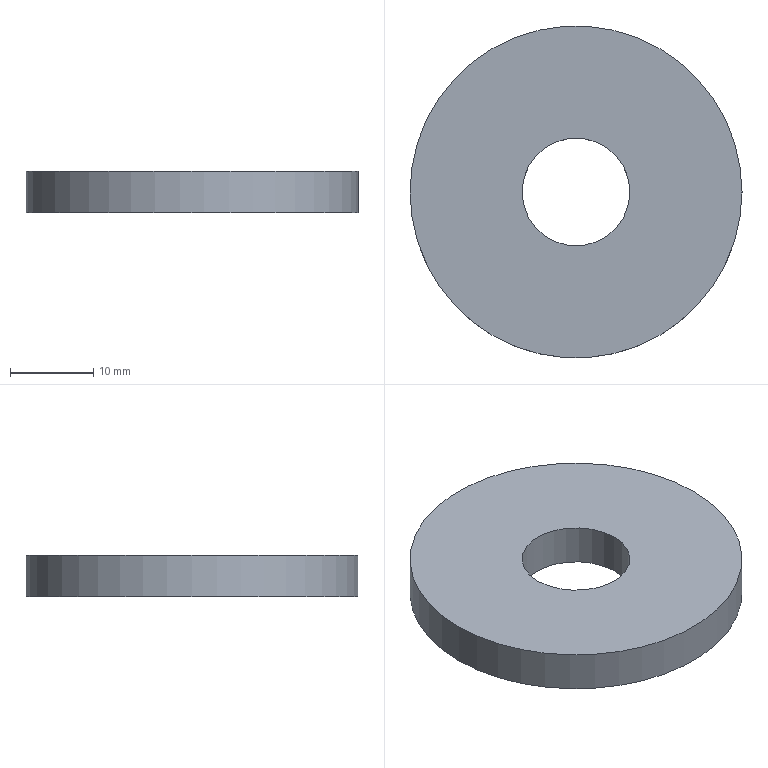Part | NX | features solid 2 | 1 solid | 4 faces | box 40 x 40 x 5 mm | volume 5620 mm3 | plane 2 | cylinder 2 | commonest cylinder face diameters 13 x1 40 x1
STEP:
#1=CARTESIAN_POINT('',(-97.5,-240.,380.));
#2=VERTEX_POINT('',#1);
#3=CARTESIAN_POINT('',(-117.5,-240.,380.));
#4=DIRECTION('',(0.,0.,1.));
#5=DIRECTION('',(1.,0.,0.));
#6=AXIS2_PLACEMENT_3D('',#3,#4,#5);
#7=CIRCLE('',#6,20.);
#8=EDGE_CURVE('',#2,#2,#7,.F.);
#9=ORIENTED_EDGE('',*,*,#8,.F.);
#10=EDGE_LOOP('',(#9));
#11=FACE_BOUND('',#10,.T.);
#12=CARTESIAN_POINT('',(-111.,-240.,380.));
#13=VERTEX_POINT('',#12);
#14=CARTESIAN_POINT('',(-117.5,-240.,380.));
#15=DIRECTION('',(0.,0.,1.));
#16=DIRECTION('',(1.,0.,0.));
#17=AXIS2_PLACEMENT_3D('',#14,#15,#16);
#18=CIRCLE('',#17,6.5);
#19=EDGE_CURVE('',#13,#13,#18,.F.);
#20=ORIENTED_EDGE('',*,*,#19,.T.);
#21=EDGE_LOOP('',(#20));
#22=FACE_BOUND('',#21,.T.);
#23=CARTESIAN_POINT('',(-117.5,-240.,380.));
#24=DIRECTION('',(0.,0.,-1.));
#25=DIRECTION('',(-1.,0.,0.));
#26=AXIS2_PLACEMENT_3D('',#23,#24,#25);
#27=PLANE('',#26);
#28=ADVANCED_FACE('',(#11,#22),#27,.F.);
#29=CARTESIAN_POINT('',(-97.5,-240.,375.));
#30=VERTEX_POINT('',#29);
#31=CARTESIAN_POINT('',(-117.5,-240.,375.));
#32=DIRECTION('',(0.,0.,1.));
#33=DIRECTION('',(1.,0.,0.));
#34=AXIS2_PLACEMENT_3D('',#31,#32,#33);
#35=CIRCLE('',#34,20.);
#36=EDGE_CURVE('',#30,#30,#35,.F.);
#37=ORIENTED_EDGE('',*,*,#36,.T.);
#38=EDGE_LOOP('',(#37));
#39=FACE_BOUND('',#38,.T.);
#40=CARTESIAN_POINT('',(-111.,-240.,375.));
#41=VERTEX_POINT('',#40);
#42=CARTESIAN_POINT('',(-117.5,-240.,375.));
#43=DIRECTION('',(0.,0.,1.));
#44=DIRECTION('',(1.,0.,0.));
#45=AXIS2_PLACEMENT_3D('',#42,#43,#44);
#46=CIRCLE('',#45,6.5);
#47=EDGE_CURVE('',#41,#41,#46,.F.);
#48=ORIENTED_EDGE('',*,*,#47,.F.);
#49=EDGE_LOOP('',(#48));
#50=FACE_BOUND('',#49,.T.);
#51=CARTESIAN_POINT('',(-117.5,-240.,375.));
#52=DIRECTION('',(0.,0.,-1.));
#53=DIRECTION('',(-1.,0.,0.));
#54=AXIS2_PLACEMENT_3D('',#51,#52,#53);
#55=PLANE('',#54);
#56=ADVANCED_FACE('',(#39,#50),#55,.T.);
#57=ORIENTED_EDGE('',*,*,#8,.T.);
#58=EDGE_LOOP('',(#57));
#59=FACE_BOUND('',#58,.T.);
#60=ORIENTED_EDGE('',*,*,#36,.F.);
#61=EDGE_LOOP('',(#60));
#62=FACE_BOUND('',#61,.T.);
#63=CARTESIAN_POINT('',(-117.5,-240.,375.));
#64=DIRECTION('',(0.,0.,1.));
#65=DIRECTION('',(1.,0.,0.));
#66=AXIS2_PLACEMENT_3D('',#63,#64,#65);
#67=CYLINDRICAL_SURFACE('',#66,20.);
#68=ADVANCED_FACE('',(#59,#62),#67,.T.);
#69=ORIENTED_EDGE('',*,*,#19,.F.);
#70=EDGE_LOOP('',(#69));
#71=FACE_BOUND('',#70,.T.);
#72=ORIENTED_EDGE('',*,*,#47,.T.);
#73=EDGE_LOOP('',(#72));
#74=FACE_BOUND('',#73,.T.);
#75=CARTESIAN_POINT('',(-117.5,-240.,375.));
#76=DIRECTION('',(0.,0.,1.));
#77=DIRECTION('',(1.,0.,0.));
#78=AXIS2_PLACEMENT_3D('',#75,#76,#77);
#79=CYLINDRICAL_SURFACE('',#78,6.5);
#80=ADVANCED_FACE('',(#71,#74),#79,.F.);
#81=CLOSED_SHELL('',(#28,#56,#68,#80));
#82=MANIFOLD_SOLID_BREP('',#81);
#83=(LENGTH_UNIT()NAMED_UNIT(*)SI_UNIT(.MILLI.,.METRE.));
#84=UNCERTAINTY_MEASURE_WITH_UNIT(LENGTH_MEASURE(0.00001),#83,'','');
#85=(NAMED_UNIT(*)PLANE_ANGLE_UNIT()SI_UNIT($,.RADIAN.));
#86=(NAMED_UNIT(*)SI_UNIT($,.STERADIAN.)SOLID_ANGLE_UNIT());
#87=(GEOMETRIC_REPRESENTATION_CONTEXT(3)GLOBAL_UNCERTAINTY_ASSIGNED_CONTEXT((#84))GLOBAL_UNIT_ASSIGNED_CONTEXT((#83,#85,#86))REPRESENTATION_CONTEXT('',''));
#88=ADVANCED_BREP_SHAPE_REPRESENTATION('',(#82),#87);